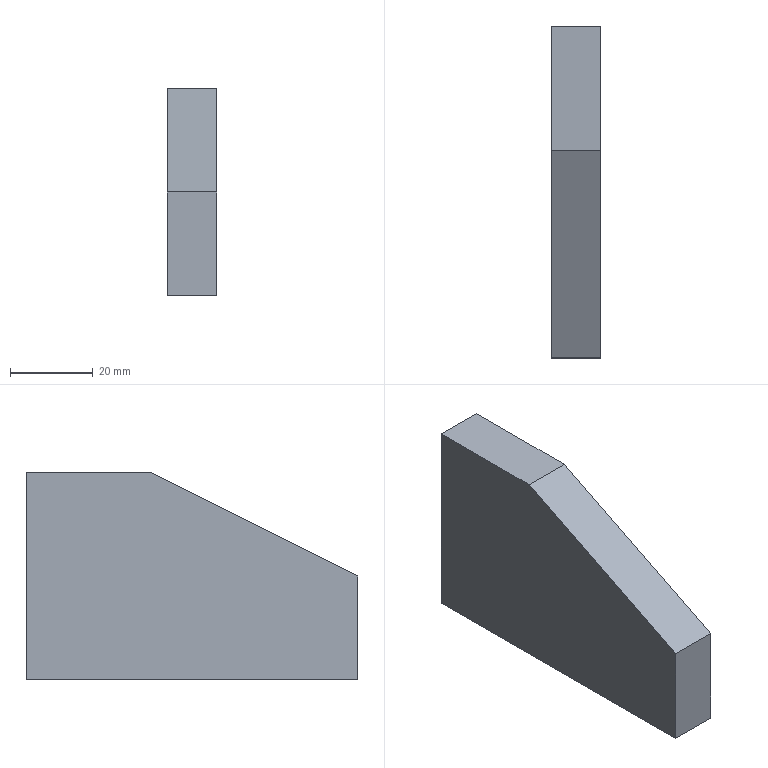Part | NX | 1 solid | 15 faces | box 12 x 80 x 50 mm | volume 39283 mm3 | plane 7 | cone 4 | cylinder 4 | commonest cylinder face diameters 5 x4
STEP:
#1=CARTESIAN_POINT('',(0.,19.5,-25.));
#2=VERTEX_POINT('',#1);
#3=CARTESIAN_POINT('',(0.,17.,-25.));
#4=DIRECTION('',(0.,0.,-1.));
#5=DIRECTION('',(0.,1.,0.));
#6=AXIS2_PLACEMENT_3D('',#3,#4,#5);
#7=CIRCLE('',#6,2.5);
#8=EDGE_CURVE('',#2,#2,#7,.T.);
#9=ORIENTED_EDGE('',*,*,#8,.F.);
#10=EDGE_LOOP('',(#9));
#11=FACE_BOUND('',#10,.T.);
#12=CARTESIAN_POINT('',(0.,-25.5,-25.));
#13=VERTEX_POINT('',#12);
#14=CARTESIAN_POINT('',(0.,-28.,-25.));
#15=DIRECTION('',(0.,0.,-1.));
#16=DIRECTION('',(0.,1.,0.));
#17=AXIS2_PLACEMENT_3D('',#14,#15,#16);
#18=CIRCLE('',#17,2.5);
#19=EDGE_CURVE('',#13,#13,#18,.T.);
#20=ORIENTED_EDGE('',*,*,#19,.F.);
#21=EDGE_LOOP('',(#20));
#22=FACE_BOUND('',#21,.T.);
#23=CARTESIAN_POINT('',(-6.,-40.,-25.));
#24=VERTEX_POINT('',#23);
#25=CARTESIAN_POINT('',(-6.,40.,-25.));
#26=VERTEX_POINT('',#25);
#27=CARTESIAN_POINT('',(-6.,40.,-25.));
#28=DIRECTION('',(0.,1.,0.));
#29=VECTOR('',#28,1000.);
#30=LINE('',#27,#29);
#31=EDGE_CURVE('',#24,#26,#30,.T.);
#32=ORIENTED_EDGE('',*,*,#31,.T.);
#33=CARTESIAN_POINT('',(6.,40.,-25.));
#34=VERTEX_POINT('',#33);
#35=CARTESIAN_POINT('',(6.,40.,-25.));
#36=DIRECTION('',(-1.,0.,0.));
#37=VECTOR('',#36,1000.);
#38=LINE('',#35,#37);
#39=EDGE_CURVE('',#34,#26,#38,.T.);
#40=ORIENTED_EDGE('',*,*,#39,.F.);
#41=CARTESIAN_POINT('',(6.,-40.,-25.));
#42=VERTEX_POINT('',#41);
#43=CARTESIAN_POINT('',(6.,40.,-25.));
#44=DIRECTION('',(0.,1.,0.));
#45=VECTOR('',#44,1000.);
#46=LINE('',#43,#45);
#47=EDGE_CURVE('',#42,#34,#46,.T.);
#48=ORIENTED_EDGE('',*,*,#47,.F.);
#49=CARTESIAN_POINT('',(6.,-40.,-25.));
#50=DIRECTION('',(-1.,0.,0.));
#51=VECTOR('',#50,1000.);
#52=LINE('',#49,#51);
#53=EDGE_CURVE('',#42,#24,#52,.T.);
#54=ORIENTED_EDGE('',*,*,#53,.T.);
#55=EDGE_LOOP('',(#32,#40,#48,#54));
#56=FACE_BOUND('',#55,.T.);
#57=CARTESIAN_POINT('',(6.,40.,-25.));
#58=DIRECTION('',(0.,0.,1.));
#59=DIRECTION('',(0.,-1.,0.));
#60=AXIS2_PLACEMENT_3D('',#57,#58,#59);
#61=PLANE('',#60);
#62=ADVANCED_FACE('',(#11,#22,#56),#61,.F.);
#63=CARTESIAN_POINT('',(0.,40.,17.5));
#64=VERTEX_POINT('',#63);
#65=CARTESIAN_POINT('',(0.,40.,15.));
#66=DIRECTION('',(0.,1.,0.));
#67=DIRECTION('',(0.,0.,1.));
#68=AXIS2_PLACEMENT_3D('',#65,#66,#67);
#69=CIRCLE('',#68,2.5);
#70=EDGE_CURVE('',#64,#64,#69,.T.);
#71=ORIENTED_EDGE('',*,*,#70,.F.);
#72=EDGE_LOOP('',(#71));
#73=FACE_BOUND('',#72,.T.);
#74=CARTESIAN_POINT('',(0.,40.,-12.5));
#75=VERTEX_POINT('',#74);
#76=CARTESIAN_POINT('',(0.,40.,-15.));
#77=DIRECTION('',(0.,1.,0.));
#78=DIRECTION('',(0.,0.,1.));
#79=AXIS2_PLACEMENT_3D('',#76,#77,#78);
#80=CIRCLE('',#79,2.5);
#81=EDGE_CURVE('',#75,#75,#80,.T.);
#82=ORIENTED_EDGE('',*,*,#81,.F.);
#83=EDGE_LOOP('',(#82));
#84=FACE_BOUND('',#83,.T.);
#85=CARTESIAN_POINT('',(-6.,40.,25.));
#86=VERTEX_POINT('',#85);
#87=CARTESIAN_POINT('',(-6.,40.,25.));
#88=DIRECTION('',(0.,0.,1.));
#89=VECTOR('',#88,1000.);
#90=LINE('',#87,#89);
#91=EDGE_CURVE('',#26,#86,#90,.T.);
#92=ORIENTED_EDGE('',*,*,#91,.T.);
#93=CARTESIAN_POINT('',(6.,40.,25.));
#94=VERTEX_POINT('',#93);
#95=CARTESIAN_POINT('',(6.,40.,25.));
#96=DIRECTION('',(-1.,0.,0.));
#97=VECTOR('',#96,1000.);
#98=LINE('',#95,#97);
#99=EDGE_CURVE('',#94,#86,#98,.T.);
#100=ORIENTED_EDGE('',*,*,#99,.F.);
#101=CARTESIAN_POINT('',(6.,40.,25.));
#102=DIRECTION('',(0.,0.,1.));
#103=VECTOR('',#102,1000.);
#104=LINE('',#101,#103);
#105=EDGE_CURVE('',#34,#94,#104,.T.);
#106=ORIENTED_EDGE('',*,*,#105,.F.);
#107=ORIENTED_EDGE('',*,*,#39,.T.);
#108=EDGE_LOOP('',(#92,#100,#106,#107));
#109=FACE_BOUND('',#108,.T.);
#110=CARTESIAN_POINT('',(6.,40.,25.));
#111=DIRECTION('',(0.,-1.,0.));
#112=DIRECTION('',(0.,0.,-1.));
#113=AXIS2_PLACEMENT_3D('',#110,#111,#112);
#114=PLANE('',#113);
#115=ADVANCED_FACE('',(#73,#84,#109),#114,.F.);
#116=CARTESIAN_POINT('',(-6.,10.,25.));
#117=VERTEX_POINT('',#116);
#118=CARTESIAN_POINT('',(-6.,40.,25.));
#119=DIRECTION('',(0.,-1.,0.));
#120=VECTOR('',#119,1000.);
#121=LINE('',#118,#120);
#122=EDGE_CURVE('',#86,#117,#121,.T.);
#123=ORIENTED_EDGE('',*,*,#122,.T.);
#124=CARTESIAN_POINT('',(6.,10.,25.));
#125=VERTEX_POINT('',#124);
#126=CARTESIAN_POINT('',(-14.,10.,25.));
#127=DIRECTION('',(1.,0.,0.));
#128=VECTOR('',#127,1000.);
#129=LINE('',#126,#128);
#130=EDGE_CURVE('',#117,#125,#129,.T.);
#131=ORIENTED_EDGE('',*,*,#130,.T.);
#132=CARTESIAN_POINT('',(6.,40.,25.));
#133=DIRECTION('',(0.,-1.,0.));
#134=VECTOR('',#133,1000.);
#135=LINE('',#132,#134);
#136=EDGE_CURVE('',#94,#125,#135,.T.);
#137=ORIENTED_EDGE('',*,*,#136,.F.);
#138=ORIENTED_EDGE('',*,*,#99,.T.);
#139=EDGE_LOOP('',(#123,#131,#137,#138));
#140=FACE_BOUND('',#139,.T.);
#141=CARTESIAN_POINT('',(6.,40.,25.));
#142=DIRECTION('',(0.,0.,-1.));
#143=DIRECTION('',(0.,1.,0.));
#144=AXIS2_PLACEMENT_3D('',#141,#142,#143);
#145=PLANE('',#144);
#146=ADVANCED_FACE('',(#140),#145,.F.);
#147=CARTESIAN_POINT('',(6.,-40.,0.));
#148=VERTEX_POINT('',#147);
#149=CARTESIAN_POINT('',(6.,-40.,25.));
#150=DIRECTION('',(0.,0.,-1.));
#151=VECTOR('',#150,1000.);
#152=LINE('',#149,#151);
#153=EDGE_CURVE('',#148,#42,#152,.T.);
#154=ORIENTED_EDGE('',*,*,#153,.F.);
#155=CARTESIAN_POINT('',(-6.,-40.,0.));
#156=VERTEX_POINT('',#155);
#157=CARTESIAN_POINT('',(-14.,-40.,0.));
#158=DIRECTION('',(1.,0.,0.));
#159=VECTOR('',#158,1000.);
#160=LINE('',#157,#159);
#161=EDGE_CURVE('',#156,#148,#160,.T.);
#162=ORIENTED_EDGE('',*,*,#161,.F.);
#163=CARTESIAN_POINT('',(-6.,-40.,25.));
#164=DIRECTION('',(0.,0.,-1.));
#165=VECTOR('',#164,1000.);
#166=LINE('',#163,#165);
#167=EDGE_CURVE('',#156,#24,#166,.T.);
#168=ORIENTED_EDGE('',*,*,#167,.T.);
#169=ORIENTED_EDGE('',*,*,#53,.F.);
#170=EDGE_LOOP('',(#154,#162,#168,#169));
#171=FACE_BOUND('',#170,.T.);
#172=CARTESIAN_POINT('',(6.,-40.,25.));
#173=DIRECTION('',(0.,1.,0.));
#174=DIRECTION('',(0.,0.,1.));
#175=AXIS2_PLACEMENT_3D('',#172,#173,#174);
#176=PLANE('',#175);
#177=ADVANCED_FACE('',(#171),#176,.F.);
#178=CARTESIAN_POINT('',(6.,-40.,0.));
#179=DIRECTION('',(0.,0.8944,0.4472));
#180=VECTOR('',#179,1000.);
#181=LINE('',#178,#180);
#182=EDGE_CURVE('',#148,#125,#181,.T.);
#183=ORIENTED_EDGE('',*,*,#182,.F.);
#184=ORIENTED_EDGE('',*,*,#153,.T.);
#185=ORIENTED_EDGE('',*,*,#47,.T.);
#186=ORIENTED_EDGE('',*,*,#105,.T.);
#187=ORIENTED_EDGE('',*,*,#136,.T.);
#188=EDGE_LOOP('',(#183,#184,#185,#186,#187));
#189=FACE_BOUND('',#188,.T.);
#190=CARTESIAN_POINT('',(6.,0.,0.));
#191=DIRECTION('',(1.,0.,0.));
#192=DIRECTION('',(0.,0.,-1.));
#193=AXIS2_PLACEMENT_3D('',#190,#191,#192);
#194=PLANE('',#193);
#195=ADVANCED_FACE('',(#189),#194,.T.);
#196=ORIENTED_EDGE('',*,*,#167,.F.);
#197=CARTESIAN_POINT('',(-6.,-8.,16.));
#198=DIRECTION('',(0.,0.8944,0.4472));
#199=VECTOR('',#198,1000.);
#200=LINE('',#197,#199);
#201=EDGE_CURVE('',#156,#117,#200,.T.);
#202=ORIENTED_EDGE('',*,*,#201,.T.);
#203=ORIENTED_EDGE('',*,*,#122,.F.);
#204=ORIENTED_EDGE('',*,*,#91,.F.);
#205=ORIENTED_EDGE('',*,*,#31,.F.);
#206=EDGE_LOOP('',(#196,#202,#203,#204,#205));
#207=FACE_BOUND('',#206,.T.);
#208=CARTESIAN_POINT('',(-6.,0.,0.));
#209=DIRECTION('',(1.,0.,0.));
#210=DIRECTION('',(0.,0.,-1.));
#211=AXIS2_PLACEMENT_3D('',#208,#209,#210);
#212=PLANE('',#211);
#213=ADVANCED_FACE('',(#207),#212,.F.);
#214=ORIENTED_EDGE('',*,*,#161,.T.);
#215=ORIENTED_EDGE('',*,*,#182,.T.);
#216=ORIENTED_EDGE('',*,*,#130,.F.);
#217=ORIENTED_EDGE('',*,*,#201,.F.);
#218=EDGE_LOOP('',(#214,#215,#216,#217));
#219=FACE_BOUND('',#218,.T.);
#220=CARTESIAN_POINT('',(-14.,-40.,0.));
#221=DIRECTION('',(0.,0.4472,-0.8944));
#222=DIRECTION('',(0.,0.8944,0.4472));
#223=AXIS2_PLACEMENT_3D('',#220,#221,#222);
#224=PLANE('',#223);
#225=ADVANCED_FACE('',(#219),#224,.F.);
#226=CARTESIAN_POINT('',(0.,-28.,-8.498));
#227=VERTEX_POINT('',#226);
#228=VERTEX_LOOP('',#227);
#229=FACE_BOUND('',#228,.T.);
#230=CARTESIAN_POINT('',(0.,-25.5,-10.));
#231=VERTEX_POINT('',#230);
#232=CARTESIAN_POINT('',(0.,-28.,-10.));
#233=DIRECTION('',(0.,0.,-1.));
#234=DIRECTION('',(0.,1.,0.));
#235=AXIS2_PLACEMENT_3D('',#232,#233,#234);
#236=CIRCLE('',#235,2.5);
#237=EDGE_CURVE('',#231,#231,#236,.T.);
#238=ORIENTED_EDGE('',*,*,#237,.T.);
#239=EDGE_LOOP('',(#238));
#240=FACE_BOUND('',#239,.T.);
#241=CARTESIAN_POINT('',(0.,-28.,-10.));
#242=DIRECTION('',(0.,0.,-1.));
#243=DIRECTION('',(0.,1.,0.));
#244=AXIS2_PLACEMENT_3D('',#241,#242,#243);
#245=CONICAL_SURFACE('',#244,2.5,1.03);
#246=ADVANCED_FACE('',(#229,#240),#245,.F.);
#247=ORIENTED_EDGE('',*,*,#237,.F.);
#248=EDGE_LOOP('',(#247));
#249=FACE_BOUND('',#248,.T.);
#250=ORIENTED_EDGE('',*,*,#19,.T.);
#251=EDGE_LOOP('',(#250));
#252=FACE_BOUND('',#251,.T.);
#253=CARTESIAN_POINT('',(0.,-28.,-25.));
#254=DIRECTION('',(0.,0.,-1.));
#255=DIRECTION('',(0.,1.,0.));
#256=AXIS2_PLACEMENT_3D('',#253,#254,#255);
#257=CYLINDRICAL_SURFACE('',#256,2.5);
#258=ADVANCED_FACE('',(#249,#252),#257,.F.);
#259=CARTESIAN_POINT('',(0.,17.,-8.498));
#260=VERTEX_POINT('',#259);
#261=VERTEX_LOOP('',#260);
#262=FACE_BOUND('',#261,.T.);
#263=CARTESIAN_POINT('',(0.,19.5,-10.));
#264=VERTEX_POINT('',#263);
#265=CARTESIAN_POINT('',(0.,17.,-10.));
#266=DIRECTION('',(0.,0.,-1.));
#267=DIRECTION('',(0.,1.,0.));
#268=AXIS2_PLACEMENT_3D('',#265,#266,#267);
#269=CIRCLE('',#268,2.5);
#270=EDGE_CURVE('',#264,#264,#269,.T.);
#271=ORIENTED_EDGE('',*,*,#270,.T.);
#272=EDGE_LOOP('',(#271));
#273=FACE_BOUND('',#272,.T.);
#274=CARTESIAN_POINT('',(0.,17.,-10.));
#275=DIRECTION('',(0.,0.,-1.));
#276=DIRECTION('',(0.,1.,0.));
#277=AXIS2_PLACEMENT_3D('',#274,#275,#276);
#278=CONICAL_SURFACE('',#277,2.5,1.03);
#279=ADVANCED_FACE('',(#262,#273),#278,.F.);
#280=ORIENTED_EDGE('',*,*,#270,.F.);
#281=EDGE_LOOP('',(#280));
#282=FACE_BOUND('',#281,.T.);
#283=ORIENTED_EDGE('',*,*,#8,.T.);
#284=EDGE_LOOP('',(#283));
#285=FACE_BOUND('',#284,.T.);
#286=CARTESIAN_POINT('',(0.,17.,-25.));
#287=DIRECTION('',(0.,0.,-1.));
#288=DIRECTION('',(0.,1.,0.));
#289=AXIS2_PLACEMENT_3D('',#286,#287,#288);
#290=CYLINDRICAL_SURFACE('',#289,2.5);
#291=ADVANCED_FACE('',(#282,#285),#290,.F.);
#292=CARTESIAN_POINT('',(0.,23.498,-15.));
#293=VERTEX_POINT('',#292);
#294=VERTEX_LOOP('',#293);
#295=FACE_BOUND('',#294,.T.);
#296=CARTESIAN_POINT('',(0.,25.,-12.5));
#297=VERTEX_POINT('',#296);
#298=CARTESIAN_POINT('',(0.,25.,-15.));
#299=DIRECTION('',(0.,1.,0.));
#300=DIRECTION('',(0.,0.,1.));
#301=AXIS2_PLACEMENT_3D('',#298,#299,#300);
#302=CIRCLE('',#301,2.5);
#303=EDGE_CURVE('',#297,#297,#302,.T.);
#304=ORIENTED_EDGE('',*,*,#303,.T.);
#305=EDGE_LOOP('',(#304));
#306=FACE_BOUND('',#305,.T.);
#307=CARTESIAN_POINT('',(0.,25.,-15.));
#308=DIRECTION('',(0.,1.,0.));
#309=DIRECTION('',(0.,0.,1.));
#310=AXIS2_PLACEMENT_3D('',#307,#308,#309);
#311=CONICAL_SURFACE('',#310,2.5,1.03);
#312=ADVANCED_FACE('',(#295,#306),#311,.F.);
#313=ORIENTED_EDGE('',*,*,#303,.F.);
#314=EDGE_LOOP('',(#313));
#315=FACE_BOUND('',#314,.T.);
#316=ORIENTED_EDGE('',*,*,#81,.T.);
#317=EDGE_LOOP('',(#316));
#318=FACE_BOUND('',#317,.T.);
#319=CARTESIAN_POINT('',(0.,40.,-15.));
#320=DIRECTION('',(0.,1.,0.));
#321=DIRECTION('',(0.,0.,1.));
#322=AXIS2_PLACEMENT_3D('',#319,#320,#321);
#323=CYLINDRICAL_SURFACE('',#322,2.5);
#324=ADVANCED_FACE('',(#315,#318),#323,.F.);
#325=CARTESIAN_POINT('',(0.,23.498,15.));
#326=VERTEX_POINT('',#325);
#327=VERTEX_LOOP('',#326);
#328=FACE_BOUND('',#327,.T.);
#329=CARTESIAN_POINT('',(0.,25.,17.5));
#330=VERTEX_POINT('',#329);
#331=CARTESIAN_POINT('',(0.,25.,15.));
#332=DIRECTION('',(0.,1.,0.));
#333=DIRECTION('',(0.,0.,1.));
#334=AXIS2_PLACEMENT_3D('',#331,#332,#333);
#335=CIRCLE('',#334,2.5);
#336=EDGE_CURVE('',#330,#330,#335,.T.);
#337=ORIENTED_EDGE('',*,*,#336,.T.);
#338=EDGE_LOOP('',(#337));
#339=FACE_BOUND('',#338,.T.);
#340=CARTESIAN_POINT('',(0.,25.,15.));
#341=DIRECTION('',(0.,1.,0.));
#342=DIRECTION('',(0.,0.,1.));
#343=AXIS2_PLACEMENT_3D('',#340,#341,#342);
#344=CONICAL_SURFACE('',#343,2.5,1.03);
#345=ADVANCED_FACE('',(#328,#339),#344,.F.);
#346=ORIENTED_EDGE('',*,*,#336,.F.);
#347=EDGE_LOOP('',(#346));
#348=FACE_BOUND('',#347,.T.);
#349=ORIENTED_EDGE('',*,*,#70,.T.);
#350=EDGE_LOOP('',(#349));
#351=FACE_BOUND('',#350,.T.);
#352=CARTESIAN_POINT('',(0.,40.,15.));
#353=DIRECTION('',(0.,1.,0.));
#354=DIRECTION('',(0.,0.,1.));
#355=AXIS2_PLACEMENT_3D('',#352,#353,#354);
#356=CYLINDRICAL_SURFACE('',#355,2.5);
#357=ADVANCED_FACE('',(#348,#351),#356,.F.);
#358=CLOSED_SHELL('',(#62,#115,#146,#177,#195,#213,#225,#246,#258,#279,#291,#312,#324,#345,#357));
#359=MANIFOLD_SOLID_BREP('',#358);
#360=(LENGTH_UNIT()NAMED_UNIT(*)SI_UNIT(.MILLI.,.METRE.));
#361=UNCERTAINTY_MEASURE_WITH_UNIT(LENGTH_MEASURE(0.00001),#360,'','');
#362=(NAMED_UNIT(*)PLANE_ANGLE_UNIT()SI_UNIT($,.RADIAN.));
#363=(NAMED_UNIT(*)SI_UNIT($,.STERADIAN.)SOLID_ANGLE_UNIT());
#364=(GEOMETRIC_REPRESENTATION_CONTEXT(3)GLOBAL_UNCERTAINTY_ASSIGNED_CONTEXT((#361))GLOBAL_UNIT_ASSIGNED_CONTEXT((#360,#362,#363))REPRESENTATION_CONTEXT('',''));
#365=ADVANCED_BREP_SHAPE_REPRESENTATION('',(#359),#364);